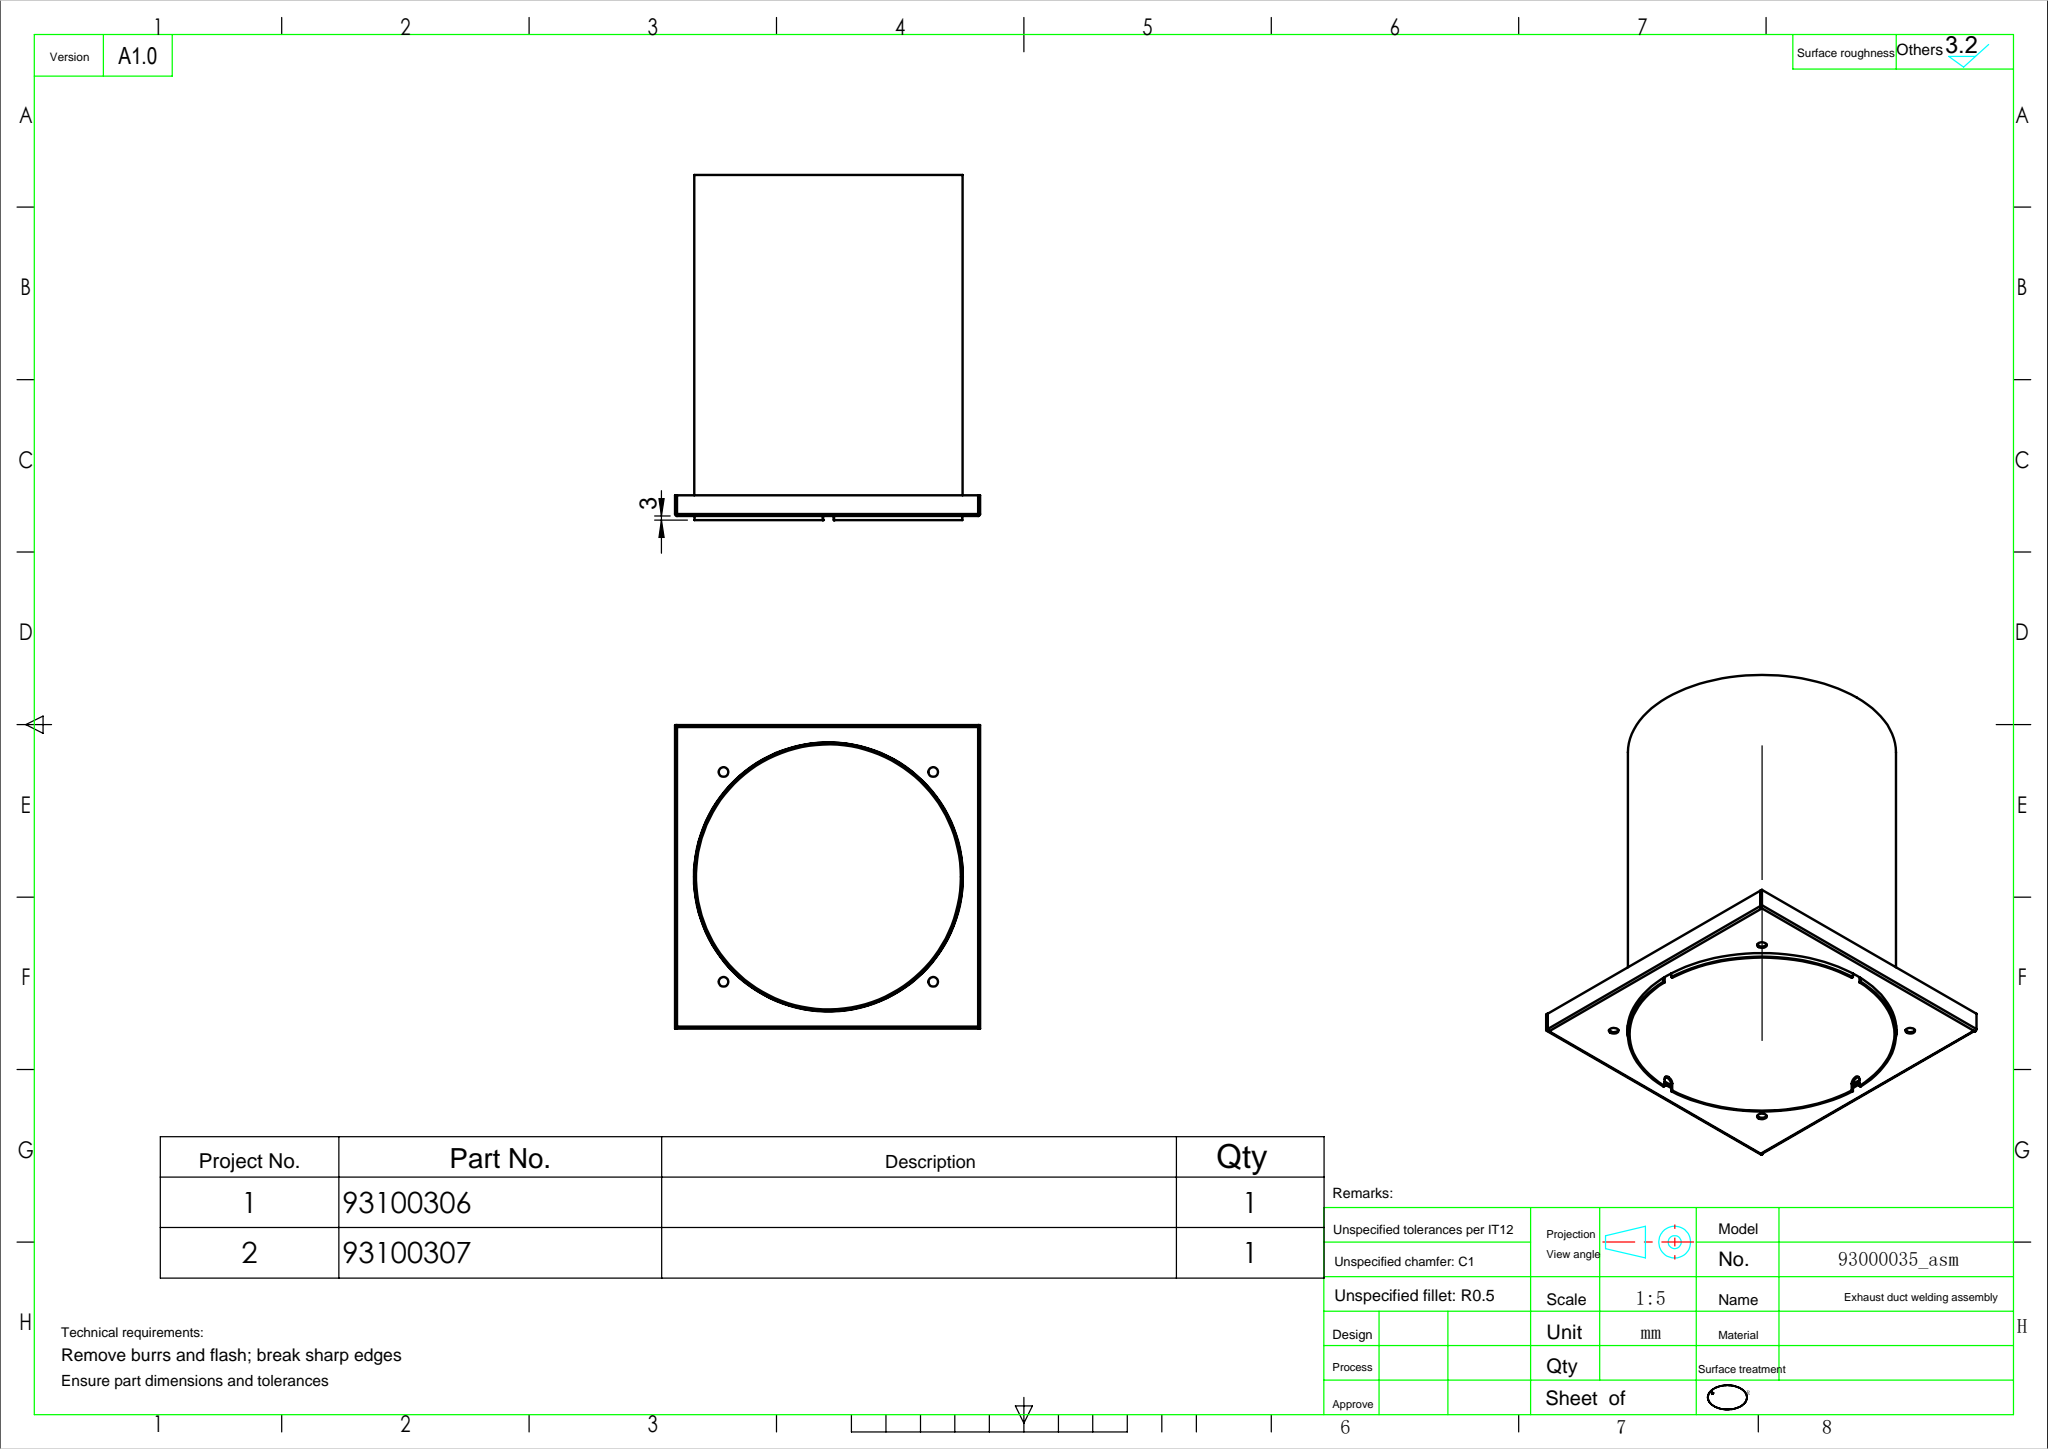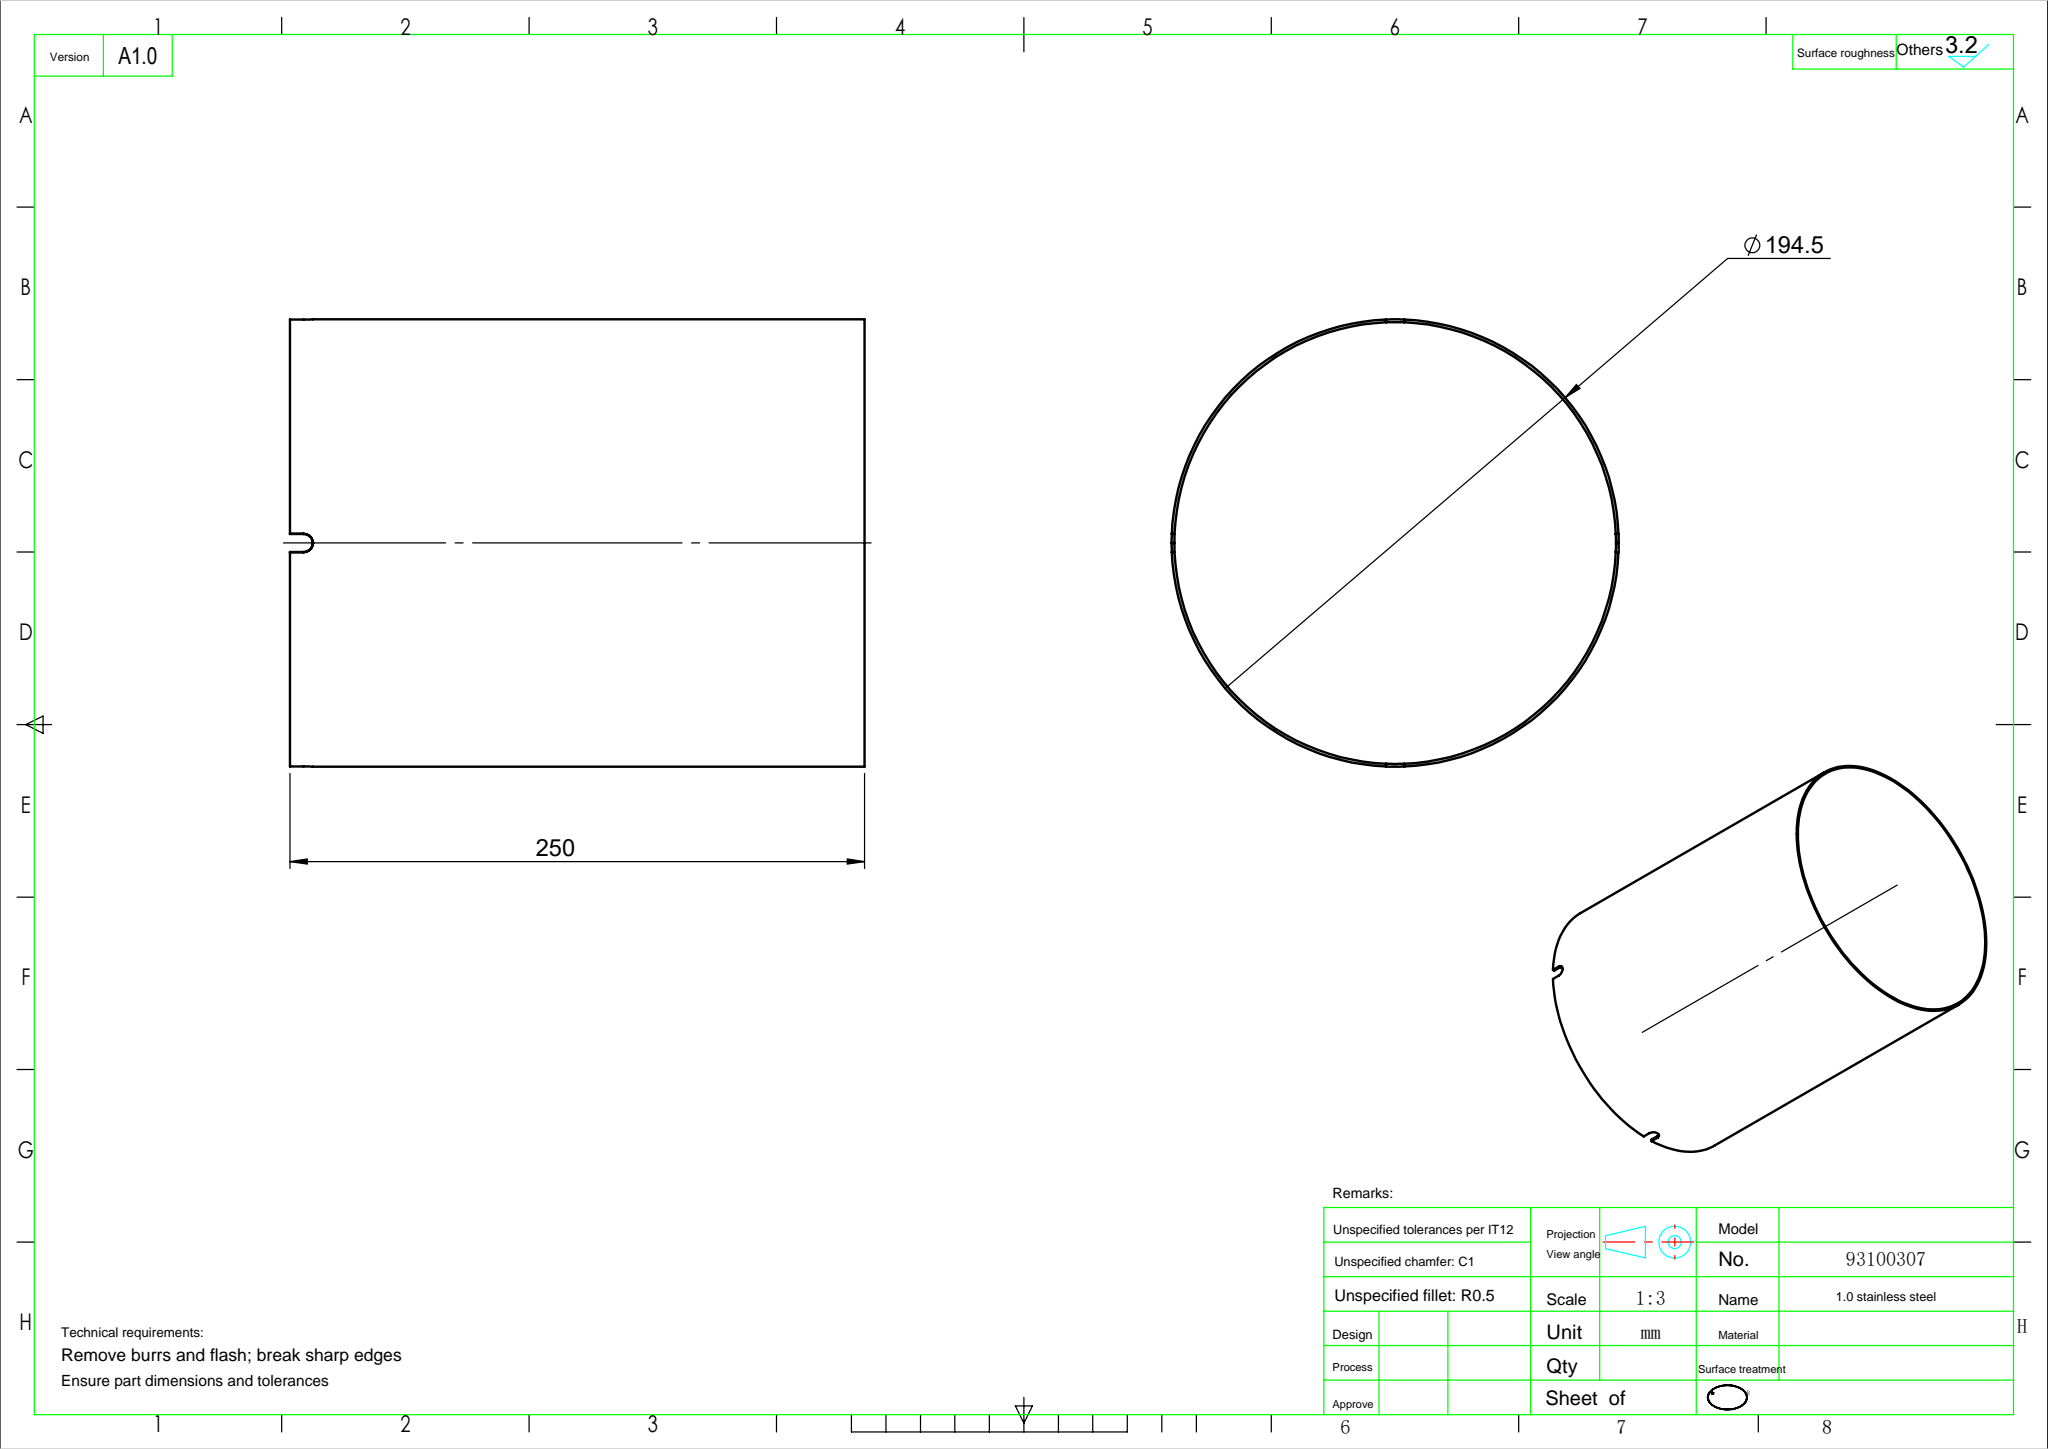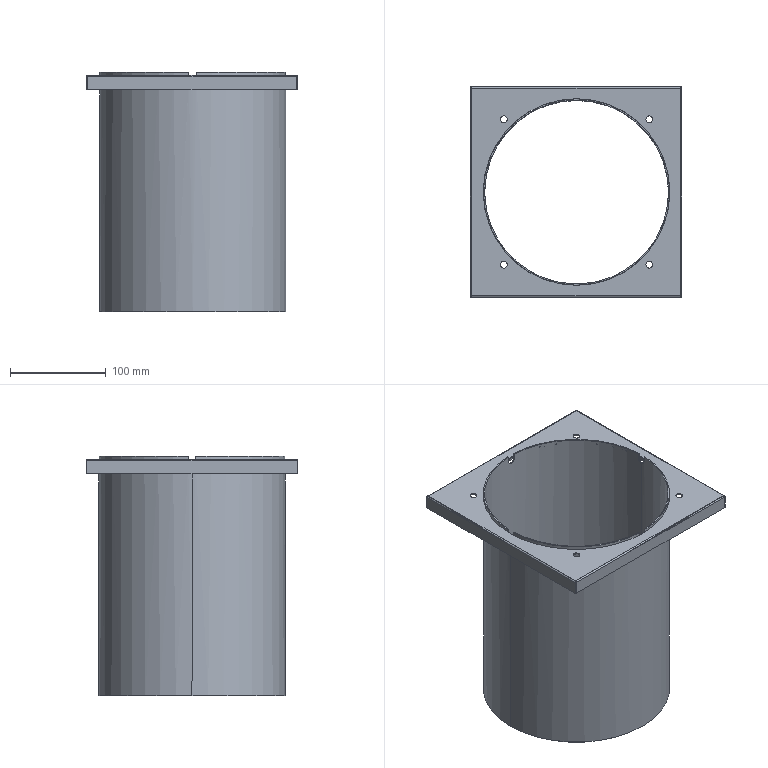Part | SolidWorks | 1 solid | 62 faces | box 221.2 x 220 x 250 mm | volume 34261 mm3 | plane 34 | cylinder 22 | spline 6 | commonest cylinder face diameters 7 x8 0.4 x4 2.8 x4 192.1 x2 194.5 x2 195 x2